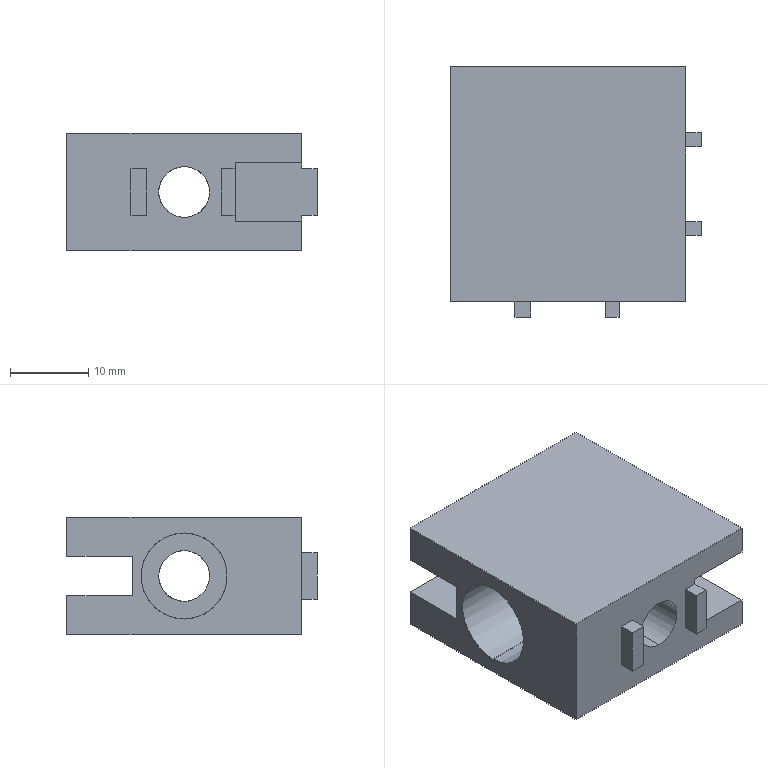Part | SolidWorks | features BaseBody 1 | 1 solid | 48 faces | box 32 x 32 x 15 mm | volume 8036 mm3 | plane 36 | cylinder 12 | commonest cylinder face diameters 11 x8 6.5 x4